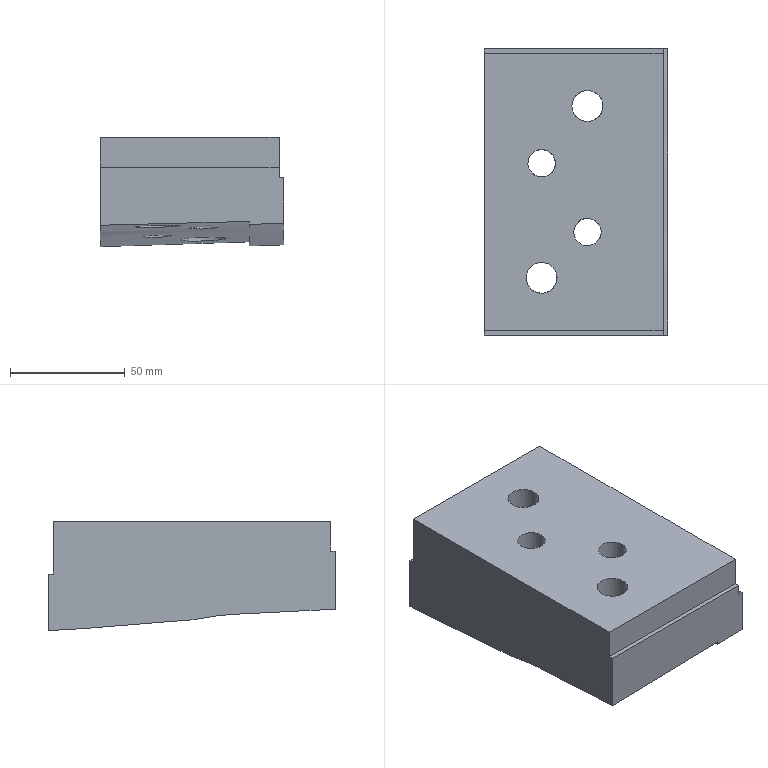Part | NX | features solid 2 | 1 solid | 22 faces | box 80 x 125 x 47.734 mm | volume 376244 mm3 | plane 9 | spline 7 | cylinder 6 | commonest cylinder face diameters 12 x2 13.5 x2 20 x2
STEP:
#1=CARTESIAN_POINT('',(-364.937,108.879,-34.001));
#2=VERTEX_POINT('',#1);
#3=CARTESIAN_POINT('',(-361.905,101.331,-33.594));
#4=CARTESIAN_POINT('',(-366.013,108.758,-34.021));
#5=CARTESIAN_POINT('',(-363.664,116.909,-34.327));
#6=CARTESIAN_POINT('',(-356.243,121.012,-34.384));
#7=CARTESIAN_POINT('',(-348.092,118.665,-34.005));
#8=CARTESIAN_POINT('',(-343.991,111.248,-33.526));
#9=CARTESIAN_POINT('',(-346.325,103.103,-33.26));
#10=CARTESIAN_POINT('',(-353.752,98.987,-33.261));
#11=CARTESIAN_POINT('',(-361.905,101.331,-33.594));
#12=CARTESIAN_POINT('',(-366.013,108.758,-34.021));
#13=CARTESIAN_POINT('',(-363.664,116.909,-34.327));
#14=B_SPLINE_CURVE_WITH_KNOTS('',3,(#3,#4,#5,#6,#7,#8,#9,#10,#11,#12,#13),.UNSPECIFIED.,.T.,.F.,(1,1,1,1,1,1,1,1,1,1,1,1,1,1,1),(-0.02346,-0.01564,-0.007821,0.,0.007821,0.01564,0.02346,0.03128,0.0391,0.04693,0.05475,0.06257,0.07039,0.07821,0.08603),.UNSPECIFIED.);
#15=EDGE_CURVE('',#2,#2,#14,.T.);
#16=ORIENTED_EDGE('',*,*,#15,.F.);
#17=EDGE_LOOP('',(#16));
#18=FACE_BOUND('',#17,.T.);
#19=CARTESIAN_POINT('',(-314.991,210.,-40.636));
#20=VERTEX_POINT('',#19);
#21=CARTESIAN_POINT('',(-314.997,85.,-31.71));
#22=VERTEX_POINT('',#21);
#23=CARTESIAN_POINT('',(-314.991,210.,-40.636));
#24=CARTESIAN_POINT('',(-314.992,204.799,-40.164));
#25=CARTESIAN_POINT('',(-314.993,196.973,-39.752));
#26=CARTESIAN_POINT('',(-314.995,186.571,-38.803));
#27=CARTESIAN_POINT('',(-314.996,176.161,-37.949));
#28=CARTESIAN_POINT('',(-314.997,163.149,-36.884));
#29=CARTESIAN_POINT('',(-314.998,147.532,-35.635));
#30=CARTESIAN_POINT('',(-314.999,131.934,-34.119));
#31=CARTESIAN_POINT('',(-314.999,116.312,-32.96));
#32=CARTESIAN_POINT('',(-314.998,100.652,-32.403));
#33=CARTESIAN_POINT('',(-314.997,90.218,-31.934));
#34=CARTESIAN_POINT('',(-314.997,85.,-31.71));
#35=B_SPLINE_CURVE_WITH_KNOTS('',3,(#23,#24,#25,#26,#27,#28,#29,#30,#31,#32,#33,#34),.UNSPECIFIED.,.F.,.F.,(4,1,1,1,1,1,1,1,1,4),(0.1412,0.1569,0.1647,0.1725,0.1882,0.2039,0.2195,0.2352,0.2508,0.2665),.UNSPECIFIED.);
#36=EDGE_CURVE('',#20,#22,#35,.T.);
#37=ORIENTED_EDGE('',*,*,#36,.T.);
#38=CARTESIAN_POINT('',(-380.,85.,-33.375));
#39=VERTEX_POINT('',#38);
#40=CARTESIAN_POINT('',(-314.997,85.,-31.71));
#41=CARTESIAN_POINT('',(-336.666,85.,-32.212));
#42=CARTESIAN_POINT('',(-358.334,85.,-32.745));
#43=CARTESIAN_POINT('',(-380.,85.,-33.375));
#44=B_SPLINE_CURVE_WITH_KNOTS('',3,(#40,#41,#42,#43),.UNSPECIFIED.,.F.,.F.,(4,4),(-0.015,0.05002),.UNSPECIFIED.);
#45=EDGE_CURVE('',#22,#39,#44,.T.);
#46=ORIENTED_EDGE('',*,*,#45,.T.);
#47=CARTESIAN_POINT('',(-380.,210.,-42.734));
#48=VERTEX_POINT('',#47);
#49=CARTESIAN_POINT('',(-380.,85.,-33.375));
#50=CARTESIAN_POINT('',(-380.,90.226,-33.532));
#51=CARTESIAN_POINT('',(-380.,98.048,-33.98));
#52=CARTESIAN_POINT('',(-380.,108.49,-34.42));
#53=CARTESIAN_POINT('',(-380.,116.32,-34.767));
#54=CARTESIAN_POINT('',(-380.,124.138,-35.273));
#55=CARTESIAN_POINT('',(-380.,130.66,-35.615));
#56=CARTESIAN_POINT('',(-380.,135.858,-36.131));
#57=CARTESIAN_POINT('',(-380.,139.738,-36.775));
#58=CARTESIAN_POINT('',(-380.,143.61,-37.525));
#59=CARTESIAN_POINT('',(-380.,148.796,-38.221));
#60=CARTESIAN_POINT('',(-380.,155.314,-38.595));
#61=CARTESIAN_POINT('',(-380.,163.121,-39.256));
#62=CARTESIAN_POINT('',(-380.,170.927,-39.912));
#63=CARTESIAN_POINT('',(-380.,178.744,-40.457));
#64=CARTESIAN_POINT('',(-380.,186.553,-41.082));
#65=CARTESIAN_POINT('',(-380.,194.346,-41.893));
#66=CARTESIAN_POINT('',(-380.,202.195,-42.062));
#67=CARTESIAN_POINT('',(-380.,207.402,-42.463));
#68=CARTESIAN_POINT('',(-380.,210.,-42.734));
#69=B_SPLINE_CURVE_WITH_KNOTS('',3,(#49,#50,#51,#52,#53,#54,#55,#56,#57,#58,#59,#60,#61,#62,#63,#64,#65,#66,#67,#68),.UNSPECIFIED.,.F.,.F.,(4,1,1,1,1,1,1,1,1,1,1,1,1,1,1,1,1,4),(0.,0.01567,0.0235,0.03134,0.03917,0.04701,0.05092,0.05484,0.05876,0.06267,0.07051,0.07834,0.08618,0.09401,0.1018,0.1097,0.1175,0.1253),.UNSPECIFIED.);
#70=EDGE_CURVE('',#39,#48,#69,.T.);
#71=ORIENTED_EDGE('',*,*,#70,.T.);
#72=CARTESIAN_POINT('',(-314.991,210.,-40.636));
#73=CARTESIAN_POINT('',(-336.664,210.,-41.245));
#74=CARTESIAN_POINT('',(-358.334,210.,-41.928));
#75=CARTESIAN_POINT('',(-380.,210.,-42.734));
#76=B_SPLINE_CURVE_WITH_KNOTS('',3,(#72,#73,#74,#75),.UNSPECIFIED.,.F.,.F.,(4,4),(0.01025,0.07529),.UNSPECIFIED.);
#77=EDGE_CURVE('',#20,#48,#76,.T.);
#78=ORIENTED_EDGE('',*,*,#77,.F.);
#79=EDGE_LOOP('',(#37,#46,#71,#78));
#80=FACE_BOUND('',#79,.T.);
#81=CARTESIAN_POINT('',(-340.6,132.154,-34.771));
#82=VERTEX_POINT('',#81);
#83=CARTESIAN_POINT('',(-337.696,136.083,-35.086));
#84=CARTESIAN_POINT('',(-341.207,132.384,-34.787));
#85=CARTESIAN_POINT('',(-341.075,127.306,-34.393));
#86=CARTESIAN_POINT('',(-337.401,123.799,-34.065));
#87=CARTESIAN_POINT('',(-332.302,123.918,-33.943));
#88=CARTESIAN_POINT('',(-328.792,127.621,-34.119));
#89=CARTESIAN_POINT('',(-328.925,132.69,-34.541));
#90=CARTESIAN_POINT('',(-332.593,136.199,-34.972));
#91=CARTESIAN_POINT('',(-337.696,136.083,-35.086));
#92=CARTESIAN_POINT('',(-341.207,132.384,-34.787));
#93=CARTESIAN_POINT('',(-341.075,127.306,-34.393));
#94=B_SPLINE_CURVE_WITH_KNOTS('',3,(#83,#84,#85,#86,#87,#88,#89,#90,#91,#92,#93),.UNSPECIFIED.,.T.,.F.,(1,1,1,1,1,1,1,1,1,1,1,1,1,1,1),(-0.01409,-0.009395,-0.004698,0.,0.004698,0.009395,0.01409,0.01879,0.02349,0.02819,0.03288,0.03758,0.04228,0.04698,0.05167),.UNSPECIFIED.);
#95=EDGE_CURVE('',#82,#82,#94,.T.);
#96=ORIENTED_EDGE('',*,*,#95,.T.);
#97=EDGE_LOOP('',(#96));
#98=FACE_BOUND('',#97,.T.);
#99=CARTESIAN_POINT('',(-360.605,162.142,-38.481));
#100=VERTEX_POINT('',#99);
#101=CARTESIAN_POINT('',(-357.704,166.08,-38.708));
#102=CARTESIAN_POINT('',(-361.214,162.37,-38.521));
#103=CARTESIAN_POINT('',(-361.069,157.294,-38.091));
#104=CARTESIAN_POINT('',(-357.392,153.797,-37.713));
#105=CARTESIAN_POINT('',(-352.294,153.921,-37.529));
#106=CARTESIAN_POINT('',(-348.787,157.631,-37.669));
#107=CARTESIAN_POINT('',(-348.93,162.701,-38.099));
#108=CARTESIAN_POINT('',(-352.604,166.202,-38.529));
#109=CARTESIAN_POINT('',(-357.704,166.08,-38.708));
#110=CARTESIAN_POINT('',(-361.214,162.37,-38.521));
#111=CARTESIAN_POINT('',(-361.069,157.294,-38.091));
#112=B_SPLINE_CURVE_WITH_KNOTS('',3,(#101,#102,#103,#104,#105,#106,#107,#108,#109,#110,#111),.UNSPECIFIED.,.T.,.F.,(1,1,1,1,1,1,1,1,1,1,1,1,1,1,1),(-0.01409,-0.009396,-0.004698,0.,0.004698,0.009396,0.01409,0.01879,0.02349,0.02819,0.03289,0.03759,0.04228,0.04698,0.05168),.UNSPECIFIED.);
#113=EDGE_CURVE('',#100,#100,#112,.T.);
#114=ORIENTED_EDGE('',*,*,#113,.T.);
#115=EDGE_LOOP('',(#114));
#116=FACE_BOUND('',#115,.T.);
#117=CARTESIAN_POINT('',(-325.058,186.077,-39.119));
#118=VERTEX_POINT('',#117);
#119=CARTESIAN_POINT('',(-328.044,193.625,-39.898));
#120=CARTESIAN_POINT('',(-323.986,186.196,-39.08));
#121=CARTESIAN_POINT('',(-326.36,178.057,-38.496));
#122=CARTESIAN_POINT('',(-333.813,173.978,-38.455));
#123=CARTESIAN_POINT('',(-341.959,176.376,-38.936));
#124=CARTESIAN_POINT('',(-346.011,183.808,-39.636));
#125=CARTESIAN_POINT('',(-343.649,191.93,-40.325));
#126=CARTESIAN_POINT('',(-336.19,196.024,-40.338));
#127=CARTESIAN_POINT('',(-328.044,193.625,-39.898));
#128=CARTESIAN_POINT('',(-323.986,186.196,-39.08));
#129=CARTESIAN_POINT('',(-326.36,178.057,-38.496));
#130=B_SPLINE_CURVE_WITH_KNOTS('',3,(#119,#120,#121,#122,#123,#124,#125,#126,#127,#128,#129),.UNSPECIFIED.,.T.,.F.,(1,1,1,1,1,1,1,1,1,1,1,1,1,1,1),(-0.02349,-0.01566,-0.007831,0.,0.007831,0.01566,0.02349,0.03133,0.03916,0.04699,0.05482,0.06265,0.07048,0.07831,0.08615),.UNSPECIFIED.);
#131=EDGE_CURVE('',#118,#118,#130,.T.);
#132=ORIENTED_EDGE('',*,*,#131,.F.);
#133=EDGE_LOOP('',(#132));
#134=FACE_BOUND('',#133,.T.);
#135=CARTESIAN_POINT('',(-307.547,210.,-40.429));
#136=CARTESIAN_POINT('',(-307.614,208.227,-40.273));
#137=CARTESIAN_POINT('',(-307.757,203.794,-39.896));
#138=CARTESIAN_POINT('',(-308.248,195.358,-39.378));
#139=CARTESIAN_POINT('',(-309.198,184.682,-38.43));
#140=CARTESIAN_POINT('',(-309.682,174.009,-37.604));
#141=CARTESIAN_POINT('',(-310.597,164.665,-36.851));
#142=CARTESIAN_POINT('',(-310.953,155.367,-36.118));
#143=CARTESIAN_POINT('',(-310.231,145.924,-35.277));
#144=CARTESIAN_POINT('',(-312.892,135.731,-34.49));
#145=CARTESIAN_POINT('',(-312.811,126.264,-33.598));
#146=CARTESIAN_POINT('',(-313.404,115.603,-32.945));
#147=CARTESIAN_POINT('',(-313.747,106.237,-32.597));
#148=CARTESIAN_POINT('',(-314.187,95.595,-32.135));
#149=CARTESIAN_POINT('',(-314.412,88.96,-31.867));
#150=CARTESIAN_POINT('',(-314.559,85.,-31.7));
#151=CARTESIAN_POINT('',(-323.481,210.,-40.865));
#152=CARTESIAN_POINT('',(-323.555,208.227,-40.703));
#153=CARTESIAN_POINT('',(-323.715,203.794,-40.315));
#154=CARTESIAN_POINT('',(-324.229,195.358,-39.951));
#155=CARTESIAN_POINT('',(-325.208,184.682,-38.945));
#156=CARTESIAN_POINT('',(-325.726,174.009,-38.166));
#157=CARTESIAN_POINT('',(-326.643,164.665,-37.425));
#158=CARTESIAN_POINT('',(-327.027,155.367,-36.673));
#159=CARTESIAN_POINT('',(-326.412,145.924,-35.93));
#160=CARTESIAN_POINT('',(-328.934,135.731,-34.777));
#161=CARTESIAN_POINT('',(-328.911,126.264,-33.989));
#162=CARTESIAN_POINT('',(-329.51,115.603,-33.326));
#163=CARTESIAN_POINT('',(-329.87,106.237,-32.976));
#164=CARTESIAN_POINT('',(-330.323,95.595,-32.512));
#165=CARTESIAN_POINT('',(-330.555,88.96,-32.226));
#166=CARTESIAN_POINT('',(-330.707,85.,-32.074));
#167=CARTESIAN_POINT('',(-347.782,210.,-41.586));
#168=CARTESIAN_POINT('',(-347.867,208.227,-41.413));
#169=CARTESIAN_POINT('',(-348.053,203.794,-41.004));
#170=CARTESIAN_POINT('',(-348.601,195.358,-40.894));
#171=CARTESIAN_POINT('',(-349.625,184.682,-39.791));
#172=CARTESIAN_POINT('',(-350.194,174.009,-39.086));
#173=CARTESIAN_POINT('',(-351.114,164.665,-38.367));
#174=CARTESIAN_POINT('',(-351.541,155.367,-37.575));
#175=CARTESIAN_POINT('',(-351.087,145.924,-37.001));
#176=CARTESIAN_POINT('',(-353.402,135.731,-35.217));
#177=CARTESIAN_POINT('',(-353.465,126.264,-34.615));
#178=CARTESIAN_POINT('',(-354.075,115.603,-33.939));
#179=CARTESIAN_POINT('',(-354.46,106.237,-33.583));
#180=CARTESIAN_POINT('',(-354.934,95.595,-33.117));
#181=CARTESIAN_POINT('',(-355.178,88.96,-32.797));
#182=CARTESIAN_POINT('',(-355.336,85.,-32.67));
#183=CARTESIAN_POINT('',(-372.07,210.,-42.438));
#184=CARTESIAN_POINT('',(-372.167,208.227,-42.259));
#185=CARTESIAN_POINT('',(-372.387,203.794,-41.833));
#186=CARTESIAN_POINT('',(-372.99,195.358,-41.776));
#187=CARTESIAN_POINT('',(-374.047,184.682,-40.655));
#188=CARTESIAN_POINT('',(-374.674,174.009,-39.963));
#189=CARTESIAN_POINT('',(-375.598,164.665,-39.253));
#190=CARTESIAN_POINT('',(-376.07,155.367,-38.433));
#191=CARTESIAN_POINT('',(-375.779,145.924,-37.966));
#192=CARTESIAN_POINT('',(-377.872,135.731,-35.815));
#193=CARTESIAN_POINT('',(-378.024,126.264,-35.342));
#194=CARTESIAN_POINT('',(-378.643,115.603,-34.667));
#195=CARTESIAN_POINT('',(-379.052,106.237,-34.301));
#196=CARTESIAN_POINT('',(-379.548,95.595,-33.828));
#197=CARTESIAN_POINT('',(-379.803,88.96,-33.482));
#198=CARTESIAN_POINT('',(-379.968,85.,-33.369));
#199=CARTESIAN_POINT('',(-380.432,210.,-42.75));
#200=CARTESIAN_POINT('',(-380.534,208.227,-42.569));
#201=CARTESIAN_POINT('',(-380.766,203.794,-42.138));
#202=CARTESIAN_POINT('',(-381.392,195.358,-42.062));
#203=CARTESIAN_POINT('',(-382.459,184.682,-40.95));
#204=CARTESIAN_POINT('',(-383.107,174.009,-40.251));
#205=CARTESIAN_POINT('',(-384.032,164.665,-39.542));
#206=CARTESIAN_POINT('',(-384.52,155.367,-38.714));
#207=CARTESIAN_POINT('',(-384.285,145.924,-38.272));
#208=CARTESIAN_POINT('',(-386.299,135.731,-36.05));
#209=CARTESIAN_POINT('',(-386.482,126.264,-35.608));
#210=CARTESIAN_POINT('',(-387.104,115.603,-34.936));
#211=CARTESIAN_POINT('',(-387.522,106.237,-34.565));
#212=CARTESIAN_POINT('',(-388.025,95.595,-34.089));
#213=CARTESIAN_POINT('',(-388.284,88.96,-33.737));
#214=CARTESIAN_POINT('',(-388.451,85.,-33.626));
#215=B_SPLINE_SURFACE_WITH_KNOTS('',3,3,((#135,#136,#137,#138,#139,#140,#141,#142,#143,#144,#145,#146,#147,#148,#149,#150),(#151,#152,#153,#154,#155,#156,#157,#158,#159,#160,#161,#162,#163,#164,#165,#166),(#167,#168,#169,#170,#171,#172,#173,#174,#175,#176,#177,#178,#179,#180,#181,#182),(#183,#184,#185,#186,#187,#188,#189,#190,#191,#192,#193,#194,#195,#196,#197,#198),(#199,#200,#201,#202,#203,#204,#205,#206,#207,#208,#209,#210,#211,#212,#213,#214)),.UNSPECIFIED.,.F.,.F.,.F.,(4,1,4),(4,1,1,1,1,1,1,1,1,1,1,1,1,4),(0.7706,0.8125,0.8345),(0.5208,0.5312,0.5469,0.5703,0.5938,0.6094,0.625,0.6484,0.6641,0.6875,0.7031,0.7266,0.7422,0.7653),.UNSPECIFIED.);
#216=ADVANCED_FACE('',(#18,#80,#98,#116,#134),#215,.F.);
#217=CARTESIAN_POINT('',(-380.,208.,5.));
#218=VERTEX_POINT('',#217);
#219=CARTESIAN_POINT('',(-380.,208.,-18.));
#220=VERTEX_POINT('',#219);
#221=CARTESIAN_POINT('',(-380.,208.,7.));
#222=DIRECTION('',(0.,0.,1.));
#223=VECTOR('',#222,1000.);
#224=LINE('',#221,#223);
#225=EDGE_CURVE('',#218,#220,#224,.F.);
#226=ORIENTED_EDGE('',*,*,#225,.T.);
#227=CARTESIAN_POINT('',(-380.,210.,-18.));
#228=VERTEX_POINT('',#227);
#229=CARTESIAN_POINT('',(-380.,210.,-18.));
#230=DIRECTION('',(0.,1.,0.));
#231=VECTOR('',#230,1000.);
#232=LINE('',#229,#231);
#233=EDGE_CURVE('',#228,#220,#232,.F.);
#234=ORIENTED_EDGE('',*,*,#233,.F.);
#235=CARTESIAN_POINT('',(-380.,210.,-24.638));
#236=DIRECTION('',(0.,0.,1.));
#237=VECTOR('',#236,1000.);
#238=LINE('',#235,#237);
#239=EDGE_CURVE('',#228,#48,#238,.F.);
#240=ORIENTED_EDGE('',*,*,#239,.T.);
#241=ORIENTED_EDGE('',*,*,#70,.F.);
#242=CARTESIAN_POINT('',(-380.,85.,-15.));
#243=VERTEX_POINT('',#242);
#244=CARTESIAN_POINT('',(-380.,85.,-33.375));
#245=CARTESIAN_POINT('',(-380.,85.,-27.25));
#246=CARTESIAN_POINT('',(-380.,85.,-21.125));
#247=CARTESIAN_POINT('',(-380.,85.,-15.));
#248=B_SPLINE_CURVE_WITH_KNOTS('',3,(#244,#245,#246,#247),.UNSPECIFIED.,.F.,.F.,(4,4),(0.,0.01837),.UNSPECIFIED.);
#249=EDGE_CURVE('',#39,#243,#248,.T.);
#250=ORIENTED_EDGE('',*,*,#249,.T.);
#251=CARTESIAN_POINT('',(-380.,85.,-8.));
#252=VERTEX_POINT('',#251);
#253=CARTESIAN_POINT('',(-380.,85.,0.505));
#254=DIRECTION('',(0.,0.,-1.));
#255=VECTOR('',#254,1000.);
#256=LINE('',#253,#255);
#257=EDGE_CURVE('',#243,#252,#256,.F.);
#258=ORIENTED_EDGE('',*,*,#257,.T.);
#259=CARTESIAN_POINT('',(-380.,87.,-8.));
#260=VERTEX_POINT('',#259);
#261=CARTESIAN_POINT('',(-380.,85.,-8.));
#262=DIRECTION('',(0.,1.,0.));
#263=VECTOR('',#262,1000.);
#264=LINE('',#261,#263);
#265=EDGE_CURVE('',#252,#260,#264,.T.);
#266=ORIENTED_EDGE('',*,*,#265,.T.);
#267=CARTESIAN_POINT('',(-380.,87.,5.));
#268=VERTEX_POINT('',#267);
#269=CARTESIAN_POINT('',(-380.,87.,12.));
#270=DIRECTION('',(0.,0.,-1.));
#271=VECTOR('',#270,1000.);
#272=LINE('',#269,#271);
#273=EDGE_CURVE('',#268,#260,#272,.T.);
#274=ORIENTED_EDGE('',*,*,#273,.F.);
#275=CARTESIAN_POINT('',(-380.,87.,5.));
#276=CARTESIAN_POINT('',(-380.,127.333,5.));
#277=CARTESIAN_POINT('',(-380.,167.667,5.));
#278=CARTESIAN_POINT('',(-380.,208.,5.));
#279=B_SPLINE_CURVE_WITH_KNOTS('',3,(#275,#276,#277,#278),.UNSPECIFIED.,.F.,.F.,(4,4),(0.1823,0.3033),.UNSPECIFIED.);
#280=EDGE_CURVE('',#268,#218,#279,.T.);
#281=ORIENTED_EDGE('',*,*,#280,.T.);
#282=EDGE_LOOP('',(#226,#234,#240,#241,#250,#258,#266,#274,#281));
#283=FACE_BOUND('',#282,.T.);
#284=CARTESIAN_POINT('',(-380.,85.,5.));
#285=CARTESIAN_POINT('',(-380.,210.,5.));
#286=CARTESIAN_POINT('',(-380.,85.,-43.02));
#287=CARTESIAN_POINT('',(-380.,210.,-43.02));
#288=B_SPLINE_SURFACE_WITH_KNOTS('',1,1,((#284,#285),(#286,#287)),.PLANE_SURF.,.F.,.F.,.F.,(2,2),(2,2),(0.3574,0.5885),(0.3333,0.4906),.PIECEWISE_BEZIER_KNOTS.);
#289=ADVANCED_FACE('',(#283),#288,.F.);
#290=CARTESIAN_POINT('',(-302.,208.,5.));
#291=VERTEX_POINT('',#290);
#292=CARTESIAN_POINT('',(-302.,208.,-18.));
#293=VERTEX_POINT('',#292);
#294=CARTESIAN_POINT('',(-302.,208.,7.));
#295=DIRECTION('',(0.,0.,1.));
#296=VECTOR('',#295,1000.);
#297=LINE('',#294,#296);
#298=EDGE_CURVE('',#291,#293,#297,.F.);
#299=ORIENTED_EDGE('',*,*,#298,.F.);
#300=CARTESIAN_POINT('',(-302.,87.,5.));
#301=VERTEX_POINT('',#300);
#302=CARTESIAN_POINT('',(-302.,87.,5.));
#303=CARTESIAN_POINT('',(-302.,127.333,5.));
#304=CARTESIAN_POINT('',(-302.,167.667,5.));
#305=CARTESIAN_POINT('',(-302.,208.,5.));
#306=B_SPLINE_CURVE_WITH_KNOTS('',3,(#302,#303,#304,#305),.UNSPECIFIED.,.F.,.F.,(4,4),(1.002,1.123),.UNSPECIFIED.);
#307=EDGE_CURVE('',#291,#301,#306,.F.);
#308=ORIENTED_EDGE('',*,*,#307,.T.);
#309=CARTESIAN_POINT('',(-302.,87.,-8.));
#310=VERTEX_POINT('',#309);
#311=CARTESIAN_POINT('',(-302.,87.,12.));
#312=DIRECTION('',(0.,0.,-1.));
#313=VECTOR('',#312,1000.);
#314=LINE('',#311,#313);
#315=EDGE_CURVE('',#301,#310,#314,.T.);
#316=ORIENTED_EDGE('',*,*,#315,.T.);
#317=CARTESIAN_POINT('',(-302.,85.,-8.));
#318=VERTEX_POINT('',#317);
#319=CARTESIAN_POINT('',(-302.,85.,-8.));
#320=DIRECTION('',(0.,1.,0.));
#321=VECTOR('',#320,1000.);
#322=LINE('',#319,#321);
#323=EDGE_CURVE('',#318,#310,#322,.T.);
#324=ORIENTED_EDGE('',*,*,#323,.F.);
#325=CARTESIAN_POINT('',(-302.,85.,-12.568));
#326=VERTEX_POINT('',#325);
#327=CARTESIAN_POINT('',(-302.,85.,-12.568));
#328=DIRECTION('',(0.,0.,1.));
#329=VECTOR('',#328,1000.);
#330=LINE('',#327,#329);
#331=EDGE_CURVE('',#326,#318,#330,.T.);
#332=ORIENTED_EDGE('',*,*,#331,.F.);
#333=CARTESIAN_POINT('',(-302.,210.,-21.967));
#334=VERTEX_POINT('',#333);
#335=CARTESIAN_POINT('',(-302.,210.,-21.967));
#336=CARTESIAN_POINT('',(-302.,168.431,-17.743));
#337=CARTESIAN_POINT('',(-302.,126.756,-14.624));
#338=CARTESIAN_POINT('',(-302.,85.,-12.568));
#339=B_SPLINE_CURVE_WITH_KNOTS('',3,(#335,#336,#337,#338),.UNSPECIFIED.,.F.,.F.,(4,4),(0.5298,1.),.UNSPECIFIED.);
#340=EDGE_CURVE('',#326,#334,#339,.F.);
#341=ORIENTED_EDGE('',*,*,#340,.T.);
#342=CARTESIAN_POINT('',(-302.,210.,-18.));
#343=VERTEX_POINT('',#342);
#344=CARTESIAN_POINT('',(-302.,210.,1.721));
#345=DIRECTION('',(0.,0.,1.));
#346=VECTOR('',#345,1000.);
#347=LINE('',#344,#346);
#348=EDGE_CURVE('',#334,#343,#347,.T.);
#349=ORIENTED_EDGE('',*,*,#348,.T.);
#350=CARTESIAN_POINT('',(-302.,210.,-18.));
#351=DIRECTION('',(0.,1.,0.));
#352=VECTOR('',#351,1000.);
#353=LINE('',#350,#352);
#354=EDGE_CURVE('',#343,#293,#353,.F.);
#355=ORIENTED_EDGE('',*,*,#354,.T.);
#356=EDGE_LOOP('',(#299,#308,#316,#324,#332,#341,#349,#355));
#357=FACE_BOUND('',#356,.T.);
#358=CARTESIAN_POINT('',(-302.,85.,-12.568));
#359=CARTESIAN_POINT('',(-302.,85.,14.357));
#360=CARTESIAN_POINT('',(-302.,126.996,-14.636));
#361=CARTESIAN_POINT('',(-302.,126.996,12.289));
#362=CARTESIAN_POINT('',(-302.,168.932,-17.78));
#363=CARTESIAN_POINT('',(-302.,168.932,9.145));
#364=CARTESIAN_POINT('',(-302.,210.748,-22.043));
#365=CARTESIAN_POINT('',(-302.,210.748,4.882));
#366=B_SPLINE_SURFACE_WITH_KNOTS('',3,1,((#358,#359),(#360,#361),(#362,#363),(#364,#365)),.SURF_OF_LINEAR_EXTRUSION.,.F.,.F.,.F.,(4,4),(2,2),(0.,0.4731),(0.,1.),.PIECEWISE_BEZIER_KNOTS.);
#367=ADVANCED_FACE('',(#357),#366,.T.);
#368=CARTESIAN_POINT('',(-341.75,185.,5.));
#369=VERTEX_POINT('',#368);
#370=CARTESIAN_POINT('',(-335.,185.,5.));
#371=DIRECTION('',(0.,0.,-1.));
#372=DIRECTION('',(-1.,0.,0.));
#373=AXIS2_PLACEMENT_3D('',#370,#371,#372);
#374=CIRCLE('',#373,6.75);
#375=EDGE_CURVE('',#369,#369,#374,.T.);
#376=ORIENTED_EDGE('',*,*,#375,.T.);
#377=EDGE_LOOP('',(#376));
#378=FACE_BOUND('',#377,.T.);
#379=CARTESIAN_POINT('',(-349.,160.,5.));
#380=VERTEX_POINT('',#379);
#381=CARTESIAN_POINT('',(-355.,160.,5.));
#382=DIRECTION('',(0.,0.,1.));
#383=DIRECTION('',(1.,0.,0.));
#384=AXIS2_PLACEMENT_3D('',#381,#382,#383);
#385=CIRCLE('',#384,6.);
#386=EDGE_CURVE('',#380,#380,#385,.F.);
#387=ORIENTED_EDGE('',*,*,#386,.T.);
#388=EDGE_LOOP('',(#387));
#389=FACE_BOUND('',#388,.T.);
#390=CARTESIAN_POINT('',(-329.,130.,5.));
#391=VERTEX_POINT('',#390);
#392=CARTESIAN_POINT('',(-335.,130.,5.));
#393=DIRECTION('',(0.,0.,1.));
#394=DIRECTION('',(1.,0.,0.));
#395=AXIS2_PLACEMENT_3D('',#392,#393,#394);
#396=CIRCLE('',#395,6.);
#397=EDGE_CURVE('',#391,#391,#396,.F.);
#398=ORIENTED_EDGE('',*,*,#397,.T.);
#399=EDGE_LOOP('',(#398));
#400=FACE_BOUND('',#399,.T.);
#401=CARTESIAN_POINT('',(-361.75,110.,5.));
#402=VERTEX_POINT('',#401);
#403=CARTESIAN_POINT('',(-355.,110.,5.));
#404=DIRECTION('',(0.,0.,-1.));
#405=DIRECTION('',(-1.,0.,0.));
#406=AXIS2_PLACEMENT_3D('',#403,#404,#405);
#407=CIRCLE('',#406,6.75);
#408=EDGE_CURVE('',#402,#402,#407,.T.);
#409=ORIENTED_EDGE('',*,*,#408,.T.);
#410=EDGE_LOOP('',(#409));
#411=FACE_BOUND('',#410,.T.);
#412=ORIENTED_EDGE('',*,*,#280,.F.);
#413=CARTESIAN_POINT('',(-302.,87.,5.));
#414=DIRECTION('',(1.,0.,0.));
#415=VECTOR('',#414,1000.);
#416=LINE('',#413,#415);
#417=EDGE_CURVE('',#301,#268,#416,.F.);
#418=ORIENTED_EDGE('',*,*,#417,.F.);
#419=ORIENTED_EDGE('',*,*,#307,.F.);
#420=CARTESIAN_POINT('',(0.,208.,5.));
#421=DIRECTION('',(1.,0.,0.));
#422=VECTOR('',#421,1000.);
#423=LINE('',#420,#422);
#424=EDGE_CURVE('',#218,#291,#423,.T.);
#425=ORIENTED_EDGE('',*,*,#424,.F.);
#426=EDGE_LOOP('',(#412,#418,#419,#425));
#427=FACE_BOUND('',#426,.T.);
#428=CARTESIAN_POINT('',(0.,0.,5.));
#429=DIRECTION('',(0.,0.,1.));
#430=DIRECTION('',(-1.,0.,0.));
#431=AXIS2_PLACEMENT_3D('',#428,#429,#430);
#432=PLANE('',#431);
#433=ADVANCED_FACE('',(#378,#389,#400,#411,#427),#432,.T.);
#434=ORIENTED_EDGE('',*,*,#348,.F.);
#435=CARTESIAN_POINT('',(-300.,210.,-21.967));
#436=VERTEX_POINT('',#435);
#437=CARTESIAN_POINT('',(-300.,210.,-21.967));
#438=CARTESIAN_POINT('',(-300.667,210.,-21.967));
#439=CARTESIAN_POINT('',(-301.333,210.,-21.967));
#440=CARTESIAN_POINT('',(-302.,210.,-21.967));
#441=B_SPLINE_CURVE_WITH_KNOTS('',3,(#437,#438,#439,#440),.UNSPECIFIED.,.F.,.F.,(4,4),(0.,0.002),.UNSPECIFIED.);
#442=EDGE_CURVE('',#436,#334,#441,.T.);
#443=ORIENTED_EDGE('',*,*,#442,.F.);
#444=CARTESIAN_POINT('',(-300.,210.,-41.967));
#445=VERTEX_POINT('',#444);
#446=CARTESIAN_POINT('',(-300.,210.,-36.492));
#447=DIRECTION('',(0.,0.,1.));
#448=VECTOR('',#447,1000.);
#449=LINE('',#446,#448);
#450=EDGE_CURVE('',#445,#436,#449,.T.);
#451=ORIENTED_EDGE('',*,*,#450,.F.);
#452=CARTESIAN_POINT('',(-314.991,210.,-42.394));
#453=VERTEX_POINT('',#452);
#454=CARTESIAN_POINT('',(-314.991,210.,-42.394));
#455=CARTESIAN_POINT('',(-309.994,210.,-42.247));
#456=CARTESIAN_POINT('',(-304.997,210.,-42.105));
#457=CARTESIAN_POINT('',(-300.,210.,-41.967));
#458=B_SPLINE_CURVE_WITH_KNOTS('',3,(#454,#455,#456,#457),.UNSPECIFIED.,.F.,.F.,(4,4),(0.0001238,0.01512),.UNSPECIFIED.);
#459=EDGE_CURVE('',#453,#445,#458,.T.);
#460=ORIENTED_EDGE('',*,*,#459,.F.);
#461=CARTESIAN_POINT('',(-314.991,210.,-46.286));
#462=DIRECTION('',(0.,0.,1.));
#463=VECTOR('',#462,1000.);
#464=LINE('',#461,#463);
#465=EDGE_CURVE('',#20,#453,#464,.F.);
#466=ORIENTED_EDGE('',*,*,#465,.F.);
#467=ORIENTED_EDGE('',*,*,#77,.T.);
#468=ORIENTED_EDGE('',*,*,#239,.F.);
#469=CARTESIAN_POINT('',(-380.,210.,-18.));
#470=DIRECTION('',(-1.,0.,0.));
#471=VECTOR('',#470,1000.);
#472=LINE('',#469,#471);
#473=EDGE_CURVE('',#228,#343,#472,.F.);
#474=ORIENTED_EDGE('',*,*,#473,.T.);
#475=EDGE_LOOP('',(#434,#443,#451,#460,#466,#467,#468,#474));
#476=FACE_BOUND('',#475,.T.);
#477=CARTESIAN_POINT('',(-130.,210.,-36.981));
#478=DIRECTION('',(0.,1.,0.));
#479=DIRECTION('',(0.,0.,1.));
#480=AXIS2_PLACEMENT_3D('',#477,#478,#479);
#481=PLANE('',#480);
#482=ADVANCED_FACE('',(#476),#481,.T.);
#483=ORIENTED_EDGE('',*,*,#450,.T.);
#484=CARTESIAN_POINT('',(-300.,85.,-12.568));
#485=VERTEX_POINT('',#484);
#486=CARTESIAN_POINT('',(-300.,85.,-12.568));
#487=CARTESIAN_POINT('',(-300.,127.002,-14.637));
#488=CARTESIAN_POINT('',(-300.,168.689,-17.77));
#489=CARTESIAN_POINT('',(-300.,210.,-21.967));
#490=B_SPLINE_CURVE_WITH_KNOTS('',3,(#486,#487,#488,#489),.UNSPECIFIED.,.F.,.F.,(4,4),(0.,0.4701),.UNSPECIFIED.);
#491=EDGE_CURVE('',#485,#436,#490,.T.);
#492=ORIENTED_EDGE('',*,*,#491,.F.);
#493=CARTESIAN_POINT('',(-300.,85.,-32.568));
#494=VERTEX_POINT('',#493);
#495=CARTESIAN_POINT('',(-300.,85.,-38.122));
#496=DIRECTION('',(0.,0.,1.));
#497=VECTOR('',#496,1000.);
#498=LINE('',#495,#497);
#499=EDGE_CURVE('',#494,#485,#498,.T.);
#500=ORIENTED_EDGE('',*,*,#499,.F.);
#501=CARTESIAN_POINT('',(-300.,85.,-32.568));
#502=CARTESIAN_POINT('',(-300.,126.745,-34.624));
#503=CARTESIAN_POINT('',(-300.,168.432,-37.743));
#504=CARTESIAN_POINT('',(-300.,210.,-41.967));
#505=B_SPLINE_CURVE_WITH_KNOTS('',3,(#501,#502,#503,#504),.UNSPECIFIED.,.F.,.F.,(4,4),(0.06289,0.1883),.UNSPECIFIED.);
#506=EDGE_CURVE('',#494,#445,#505,.T.);
#507=ORIENTED_EDGE('',*,*,#506,.T.);
#508=EDGE_LOOP('',(#483,#492,#500,#507));
#509=FACE_BOUND('',#508,.T.);
#510=CARTESIAN_POINT('',(-300.,210.,-42.143));
#511=CARTESIAN_POINT('',(-300.,210.,-12.391));
#512=CARTESIAN_POINT('',(-300.,168.426,-42.143));
#513=CARTESIAN_POINT('',(-300.,168.426,-12.391));
#514=CARTESIAN_POINT('',(-300.,126.739,-42.143));
#515=CARTESIAN_POINT('',(-300.,126.739,-12.391));
#516=CARTESIAN_POINT('',(-300.,85.,-42.143));
#517=CARTESIAN_POINT('',(-300.,85.,-12.391));
#518=B_SPLINE_SURFACE_WITH_KNOTS('',3,1,((#510,#511),(#512,#513),(#514,#515),(#516,#517)),.SURF_OF_LINEAR_EXTRUSION.,.F.,.F.,.F.,(4,4),(2,2),(0.8271,0.9135),(0.,1.),.PIECEWISE_BEZIER_KNOTS.);
#519=ADVANCED_FACE('',(#509),#518,.F.);
#520=ORIENTED_EDGE('',*,*,#459,.T.);
#521=ORIENTED_EDGE('',*,*,#506,.F.);
#522=CARTESIAN_POINT('',(-314.997,85.,-32.983));
#523=VERTEX_POINT('',#522);
#524=CARTESIAN_POINT('',(-314.997,85.,-32.983));
#525=CARTESIAN_POINT('',(-309.998,85.,-32.841));
#526=CARTESIAN_POINT('',(-304.999,85.,-32.702));
#527=CARTESIAN_POINT('',(-300.,85.,-32.568));
#528=B_SPLINE_CURVE_WITH_KNOTS('',3,(#524,#525,#526,#527),.UNSPECIFIED.,.F.,.F.,(4,4),(0.02533,0.04034),.UNSPECIFIED.);
#529=EDGE_CURVE('',#523,#494,#528,.T.);
#530=ORIENTED_EDGE('',*,*,#529,.F.);
#531=CARTESIAN_POINT('',(-314.991,210.,-42.394));
#532=CARTESIAN_POINT('',(-314.999,168.428,-38.165));
#533=CARTESIAN_POINT('',(-315.001,126.743,-35.043));
#534=CARTESIAN_POINT('',(-314.997,85.,-32.983));
#535=B_SPLINE_CURVE_WITH_KNOTS('',3,(#531,#532,#533,#534),.UNSPECIFIED.,.F.,.F.,(4,4),(0.1412,0.2666),.UNSPECIFIED.);
#536=EDGE_CURVE('',#453,#523,#535,.T.);
#537=ORIENTED_EDGE('',*,*,#536,.F.);
#538=EDGE_LOOP('',(#520,#521,#530,#537));
#539=FACE_BOUND('',#538,.T.);
#540=CARTESIAN_POINT('',(-315.081,210.804,-42.478));
#541=CARTESIAN_POINT('',(-311.281,210.791,-42.365));
#542=CARTESIAN_POINT('',(-307.481,210.777,-42.255));
#543=CARTESIAN_POINT('',(-303.681,210.764,-42.146));
#544=CARTESIAN_POINT('',(-299.881,210.752,-42.04));
#545=CARTESIAN_POINT('',(-315.088,179.092,-39.242));
#546=CARTESIAN_POINT('',(-311.287,179.079,-39.13));
#547=CARTESIAN_POINT('',(-307.487,179.066,-39.02));
#548=CARTESIAN_POINT('',(-303.687,179.053,-38.913));
#549=CARTESIAN_POINT('',(-299.887,179.04,-38.807));
#550=CARTESIAN_POINT('',(-315.094,147.436,-36.586));
#551=CARTESIAN_POINT('',(-311.294,147.422,-36.475));
#552=CARTESIAN_POINT('',(-307.494,147.409,-36.366));
#553=CARTESIAN_POINT('',(-303.694,147.397,-36.26));
#554=CARTESIAN_POINT('',(-299.894,147.384,-36.156));
#555=CARTESIAN_POINT('',(-315.102,115.825,-34.498));
#556=CARTESIAN_POINT('',(-311.302,115.812,-34.388));
#557=CARTESIAN_POINT('',(-307.501,115.799,-34.28));
#558=CARTESIAN_POINT('',(-303.701,115.787,-34.174));
#559=CARTESIAN_POINT('',(-299.901,115.774,-34.071));
#560=CARTESIAN_POINT('',(-315.112,84.252,-32.95));
#561=CARTESIAN_POINT('',(-311.311,84.239,-32.841));
#562=CARTESIAN_POINT('',(-307.511,84.226,-32.734));
#563=CARTESIAN_POINT('',(-303.711,84.213,-32.629));
#564=CARTESIAN_POINT('',(-299.91,84.201,-32.526));
#565=B_SPLINE_SURFACE_WITH_KNOTS('',4,4,((#540,#541,#542,#543,#544),(#545,#546,#547,#548,#549),(#550,#551,#552,#553,#554),(#555,#556,#557,#558,#559),(#560,#561,#562,#563,#564)),.UNSPECIFIED.,.F.,.F.,.F.,(5,5),(5,5),(0.5175,0.7103),(0.4164,0.4349),.PIECEWISE_BEZIER_KNOTS.);
#566=ADVANCED_FACE('',(#539),#565,.F.);
#567=ORIENTED_EDGE('',*,*,#442,.T.);
#568=ORIENTED_EDGE('',*,*,#340,.F.);
#569=CARTESIAN_POINT('',(-302.,85.,-12.568));
#570=CARTESIAN_POINT('',(-301.333,85.,-12.568));
#571=CARTESIAN_POINT('',(-300.667,85.,-12.568));
#572=CARTESIAN_POINT('',(-300.,85.,-12.568));
#573=B_SPLINE_CURVE_WITH_KNOTS('',3,(#569,#570,#571,#572),.UNSPECIFIED.,.F.,.F.,(4,4),(0.,1.),.UNSPECIFIED.);
#574=EDGE_CURVE('',#485,#326,#573,.F.);
#575=ORIENTED_EDGE('',*,*,#574,.F.);
#576=ORIENTED_EDGE('',*,*,#491,.T.);
#577=EDGE_LOOP('',(#567,#568,#575,#576));
#578=FACE_BOUND('',#577,.T.);
#579=CARTESIAN_POINT('',(-302.,85.,-12.568));
#580=CARTESIAN_POINT('',(-302.,126.756,-14.624));
#581=CARTESIAN_POINT('',(-302.,168.431,-17.743));
#582=CARTESIAN_POINT('',(-302.,210.,-21.967));
#583=CARTESIAN_POINT('',(-300.,85.,-12.568));
#584=CARTESIAN_POINT('',(-300.,126.756,-14.624));
#585=CARTESIAN_POINT('',(-300.,168.431,-17.743));
#586=CARTESIAN_POINT('',(-300.,210.,-21.967));
#587=B_SPLINE_SURFACE_WITH_KNOTS('',1,3,((#579,#580,#581,#582),(#583,#584,#585,#586)),.SURF_OF_LINEAR_EXTRUSION.,.F.,.F.,.F.,(2,2),(4,4),(0.,1.),(0.,0.4702),.PIECEWISE_BEZIER_KNOTS.);
#588=ADVANCED_FACE('',(#578),#587,.T.);
#589=ORIENTED_EDGE('',*,*,#465,.T.);
#590=ORIENTED_EDGE('',*,*,#536,.T.);
#591=CARTESIAN_POINT('',(-314.997,85.,-46.));
#592=DIRECTION('',(0.,0.,1.));
#593=VECTOR('',#592,1000.);
#594=LINE('',#591,#593);
#595=EDGE_CURVE('',#523,#22,#594,.T.);
#596=ORIENTED_EDGE('',*,*,#595,.T.);
#597=ORIENTED_EDGE('',*,*,#36,.F.);
#598=EDGE_LOOP('',(#589,#590,#596,#597));
#599=FACE_BOUND('',#598,.T.);
#600=CARTESIAN_POINT('',(-314.997,85.,-42.458));
#601=CARTESIAN_POINT('',(-314.997,85.,-31.646));
#602=CARTESIAN_POINT('',(-315.001,124.945,-42.458));
#603=CARTESIAN_POINT('',(-315.001,124.945,-31.646));
#604=CARTESIAN_POINT('',(-314.999,166.611,-42.458));
#605=CARTESIAN_POINT('',(-314.999,166.611,-31.646));
#606=CARTESIAN_POINT('',(-314.991,210.,-42.458));
#607=CARTESIAN_POINT('',(-314.991,210.,-31.646));
#608=B_SPLINE_SURFACE_WITH_KNOTS('',3,1,((#600,#601),(#602,#603),(#604,#605),(#606,#607)),.SURF_OF_LINEAR_EXTRUSION.,.F.,.F.,.F.,(4,4),(2,2),(-0.0000028,0.4728),(0.,1.),.PIECEWISE_BEZIER_KNOTS.);
#609=ADVANCED_FACE('',(#599),#608,.F.);
#610=ORIENTED_EDGE('',*,*,#417,.T.);
#611=ORIENTED_EDGE('',*,*,#273,.T.);
#612=CARTESIAN_POINT('',(-302.,87.,-8.));
#613=DIRECTION('',(-1.,0.,0.));
#614=VECTOR('',#613,1000.);
#615=LINE('',#612,#614);
#616=EDGE_CURVE('',#310,#260,#615,.T.);
#617=ORIENTED_EDGE('',*,*,#616,.F.);
#618=ORIENTED_EDGE('',*,*,#315,.F.);
#619=EDGE_LOOP('',(#610,#611,#617,#618));
#620=FACE_BOUND('',#619,.T.);
#621=CARTESIAN_POINT('',(-302.,87.,12.));
#622=DIRECTION('',(0.,-1.,0.));
#623=DIRECTION('',(-1.,0.,0.));
#624=AXIS2_PLACEMENT_3D('',#621,#622,#623);
#625=PLANE('',#624);
#626=ADVANCED_FACE('',(#620),#625,.T.);
#627=ORIENTED_EDGE('',*,*,#331,.T.);
#628=CARTESIAN_POINT('',(-302.,85.,-8.));
#629=DIRECTION('',(-1.,0.,0.));
#630=VECTOR('',#629,1000.);
#631=LINE('',#628,#630);
#632=EDGE_CURVE('',#318,#252,#631,.T.);
#633=ORIENTED_EDGE('',*,*,#632,.T.);
#634=ORIENTED_EDGE('',*,*,#257,.F.);
#635=ORIENTED_EDGE('',*,*,#249,.F.);
#636=ORIENTED_EDGE('',*,*,#45,.F.);
#637=ORIENTED_EDGE('',*,*,#595,.F.);
#638=ORIENTED_EDGE('',*,*,#529,.T.);
#639=ORIENTED_EDGE('',*,*,#499,.T.);
#640=ORIENTED_EDGE('',*,*,#574,.T.);
#641=EDGE_LOOP('',(#627,#633,#634,#635,#636,#637,#638,#639,#640));
#642=FACE_BOUND('',#641,.T.);
#643=CARTESIAN_POINT('',(412.414,85.,0.505));
#644=DIRECTION('',(0.,1.,0.));
#645=DIRECTION('',(0.,0.,1.));
#646=AXIS2_PLACEMENT_3D('',#643,#644,#645);
#647=PLANE('',#646);
#648=ADVANCED_FACE('',(#642),#647,.F.);
#649=ORIENTED_EDGE('',*,*,#616,.T.);
#650=ORIENTED_EDGE('',*,*,#265,.F.);
#651=ORIENTED_EDGE('',*,*,#632,.F.);
#652=ORIENTED_EDGE('',*,*,#323,.T.);
#653=EDGE_LOOP('',(#649,#650,#651,#652));
#654=FACE_BOUND('',#653,.T.);
#655=CARTESIAN_POINT('',(-302.,85.,-8.));
#656=DIRECTION('',(0.,0.,-1.));
#657=DIRECTION('',(-1.,0.,0.));
#658=AXIS2_PLACEMENT_3D('',#655,#656,#657);
#659=PLANE('',#658);
#660=ADVANCED_FACE('',(#654),#659,.F.);
#661=ORIENTED_EDGE('',*,*,#298,.T.);
#662=CARTESIAN_POINT('',(-380.,208.,-18.));
#663=DIRECTION('',(-1.,0.,0.));
#664=VECTOR('',#663,1000.);
#665=LINE('',#662,#664);
#666=EDGE_CURVE('',#220,#293,#665,.F.);
#667=ORIENTED_EDGE('',*,*,#666,.F.);
#668=ORIENTED_EDGE('',*,*,#225,.F.);
#669=ORIENTED_EDGE('',*,*,#424,.T.);
#670=EDGE_LOOP('',(#661,#667,#668,#669));
#671=FACE_BOUND('',#670,.T.);
#672=CARTESIAN_POINT('',(-380.,208.,7.));
#673=DIRECTION('',(0.,1.,0.));
#674=DIRECTION('',(1.,0.,0.));
#675=AXIS2_PLACEMENT_3D('',#672,#673,#674);
#676=PLANE('',#675);
#677=ADVANCED_FACE('',(#671),#676,.T.);
#678=ORIENTED_EDGE('',*,*,#666,.T.);
#679=ORIENTED_EDGE('',*,*,#354,.F.);
#680=ORIENTED_EDGE('',*,*,#473,.F.);
#681=ORIENTED_EDGE('',*,*,#233,.T.);
#682=EDGE_LOOP('',(#678,#679,#680,#681));
#683=FACE_BOUND('',#682,.T.);
#684=CARTESIAN_POINT('',(-380.,210.,-18.));
#685=DIRECTION('',(0.,0.,1.));
#686=DIRECTION('',(-1.,0.,0.));
#687=AXIS2_PLACEMENT_3D('',#684,#685,#686);
#688=PLANE('',#687);
#689=ADVANCED_FACE('',(#683),#688,.T.);
#690=ORIENTED_EDGE('',*,*,#15,.T.);
#691=EDGE_LOOP('',(#690));
#692=FACE_BOUND('',#691,.T.);
#693=CARTESIAN_POINT('',(-355.,120.,-10.));
#694=VERTEX_POINT('',#693);
#695=CARTESIAN_POINT('',(-355.,110.,-10.));
#696=DIRECTION('',(0.,0.,1.));
#697=DIRECTION('',(0.,1.,0.));
#698=AXIS2_PLACEMENT_3D('',#695,#696,#697);
#699=CIRCLE('',#698,10.);
#700=EDGE_CURVE('',#694,#694,#699,.T.);
#701=ORIENTED_EDGE('',*,*,#700,.T.);
#702=EDGE_LOOP('',(#701));
#703=FACE_BOUND('',#702,.T.);
#704=CARTESIAN_POINT('',(-355.,110.,-120.));
#705=DIRECTION('',(0.,0.,1.));
#706=DIRECTION('',(-1.,0.,0.));
#707=AXIS2_PLACEMENT_3D('',#704,#705,#706);
#708=CYLINDRICAL_SURFACE('',#707,10.);
#709=ADVANCED_FACE('',(#692,#703),#708,.F.);
#710=CARTESIAN_POINT('',(-355.,116.75,-10.));
#711=VERTEX_POINT('',#710);
#712=CARTESIAN_POINT('',(-355.,110.,-10.));
#713=DIRECTION('',(0.,0.,1.));
#714=DIRECTION('',(0.,1.,0.));
#715=AXIS2_PLACEMENT_3D('',#712,#713,#714);
#716=CIRCLE('',#715,6.75);
#717=EDGE_CURVE('',#711,#711,#716,.T.);
#718=ORIENTED_EDGE('',*,*,#717,.T.);
#719=EDGE_LOOP('',(#718));
#720=FACE_BOUND('',#719,.T.);
#721=ORIENTED_EDGE('',*,*,#700,.F.);
#722=EDGE_LOOP('',(#721));
#723=FACE_BOUND('',#722,.T.);
#724=CARTESIAN_POINT('',(-355.,110.,-10.));
#725=DIRECTION('',(0.,0.,-1.));
#726=DIRECTION('',(0.,1.,0.));
#727=AXIS2_PLACEMENT_3D('',#724,#725,#726);
#728=PLANE('',#727);
#729=ADVANCED_FACE('',(#720,#723),#728,.T.);
#730=ORIENTED_EDGE('',*,*,#408,.F.);
#731=EDGE_LOOP('',(#730));
#732=FACE_BOUND('',#731,.T.);
#733=ORIENTED_EDGE('',*,*,#717,.F.);
#734=EDGE_LOOP('',(#733));
#735=FACE_BOUND('',#734,.T.);
#736=CARTESIAN_POINT('',(-355.,110.,-95.));
#737=DIRECTION('',(0.,0.,1.));
#738=DIRECTION('',(-1.,0.,0.));
#739=AXIS2_PLACEMENT_3D('',#736,#737,#738);
#740=CYLINDRICAL_SURFACE('',#739,6.75);
#741=ADVANCED_FACE('',(#732,#735),#740,.F.);
#742=ORIENTED_EDGE('',*,*,#95,.F.);
#743=EDGE_LOOP('',(#742));
#744=FACE_BOUND('',#743,.T.);
#745=ORIENTED_EDGE('',*,*,#397,.F.);
#746=EDGE_LOOP('',(#745));
#747=FACE_BOUND('',#746,.T.);
#748=CARTESIAN_POINT('',(-335.,130.,-195.));
#749=DIRECTION('',(0.,0.,1.));
#750=DIRECTION('',(-1.,0.,0.));
#751=AXIS2_PLACEMENT_3D('',#748,#749,#750);
#752=CYLINDRICAL_SURFACE('',#751,6.);
#753=ADVANCED_FACE('',(#744,#747),#752,.F.);
#754=ORIENTED_EDGE('',*,*,#113,.F.);
#755=EDGE_LOOP('',(#754));
#756=FACE_BOUND('',#755,.T.);
#757=ORIENTED_EDGE('',*,*,#386,.F.);
#758=EDGE_LOOP('',(#757));
#759=FACE_BOUND('',#758,.T.);
#760=CARTESIAN_POINT('',(-355.,160.,-195.));
#761=DIRECTION('',(0.,0.,1.));
#762=DIRECTION('',(-1.,0.,0.));
#763=AXIS2_PLACEMENT_3D('',#760,#761,#762);
#764=CYLINDRICAL_SURFACE('',#763,6.);
#765=ADVANCED_FACE('',(#756,#759),#764,.F.);
#766=ORIENTED_EDGE('',*,*,#131,.T.);
#767=EDGE_LOOP('',(#766));
#768=FACE_BOUND('',#767,.T.);
#769=CARTESIAN_POINT('',(-335.,195.,-10.));
#770=VERTEX_POINT('',#769);
#771=CARTESIAN_POINT('',(-335.,185.,-10.));
#772=DIRECTION('',(0.,0.,1.));
#773=DIRECTION('',(0.,1.,0.));
#774=AXIS2_PLACEMENT_3D('',#771,#772,#773);
#775=CIRCLE('',#774,10.);
#776=EDGE_CURVE('',#770,#770,#775,.T.);
#777=ORIENTED_EDGE('',*,*,#776,.T.);
#778=EDGE_LOOP('',(#777));
#779=FACE_BOUND('',#778,.T.);
#780=CARTESIAN_POINT('',(-335.,185.,-120.));
#781=DIRECTION('',(0.,0.,1.));
#782=DIRECTION('',(-1.,0.,0.));
#783=AXIS2_PLACEMENT_3D('',#780,#781,#782);
#784=CYLINDRICAL_SURFACE('',#783,10.);
#785=ADVANCED_FACE('',(#768,#779),#784,.F.);
#786=CARTESIAN_POINT('',(-335.,191.75,-10.));
#787=VERTEX_POINT('',#786);
#788=CARTESIAN_POINT('',(-335.,185.,-10.));
#789=DIRECTION('',(0.,0.,1.));
#790=DIRECTION('',(0.,1.,0.));
#791=AXIS2_PLACEMENT_3D('',#788,#789,#790);
#792=CIRCLE('',#791,6.75);
#793=EDGE_CURVE('',#787,#787,#792,.T.);
#794=ORIENTED_EDGE('',*,*,#793,.T.);
#795=EDGE_LOOP('',(#794));
#796=FACE_BOUND('',#795,.T.);
#797=ORIENTED_EDGE('',*,*,#776,.F.);
#798=EDGE_LOOP('',(#797));
#799=FACE_BOUND('',#798,.T.);
#800=CARTESIAN_POINT('',(-335.,185.,-10.));
#801=DIRECTION('',(0.,0.,-1.));
#802=DIRECTION('',(0.,1.,0.));
#803=AXIS2_PLACEMENT_3D('',#800,#801,#802);
#804=PLANE('',#803);
#805=ADVANCED_FACE('',(#796,#799),#804,.T.);
#806=ORIENTED_EDGE('',*,*,#375,.F.);
#807=EDGE_LOOP('',(#806));
#808=FACE_BOUND('',#807,.T.);
#809=ORIENTED_EDGE('',*,*,#793,.F.);
#810=EDGE_LOOP('',(#809));
#811=FACE_BOUND('',#810,.T.);
#812=CARTESIAN_POINT('',(-335.,185.,-95.));
#813=DIRECTION('',(0.,0.,1.));
#814=DIRECTION('',(-1.,0.,0.));
#815=AXIS2_PLACEMENT_3D('',#812,#813,#814);
#816=CYLINDRICAL_SURFACE('',#815,6.75);
#817=ADVANCED_FACE('',(#808,#811),#816,.F.);
#818=CLOSED_SHELL('',(#216,#289,#367,#433,#482,#519,#566,#588,#609,#626,#648,#660,#677,#689,#709,#729,#741,#753,#765,#785,#805,#817));
#819=MANIFOLD_SOLID_BREP('',#818);
#820=(LENGTH_UNIT()NAMED_UNIT(*)SI_UNIT(.MILLI.,.METRE.));
#821=UNCERTAINTY_MEASURE_WITH_UNIT(LENGTH_MEASURE(0.0508),#820,'','');
#822=(NAMED_UNIT(*)PLANE_ANGLE_UNIT()SI_UNIT($,.RADIAN.));
#823=(NAMED_UNIT(*)SI_UNIT($,.STERADIAN.)SOLID_ANGLE_UNIT());
#824=(GEOMETRIC_REPRESENTATION_CONTEXT(3)GLOBAL_UNCERTAINTY_ASSIGNED_CONTEXT((#821))GLOBAL_UNIT_ASSIGNED_CONTEXT((#820,#822,#823))REPRESENTATION_CONTEXT('',''));
#825=ADVANCED_BREP_SHAPE_REPRESENTATION('',(#819),#824);